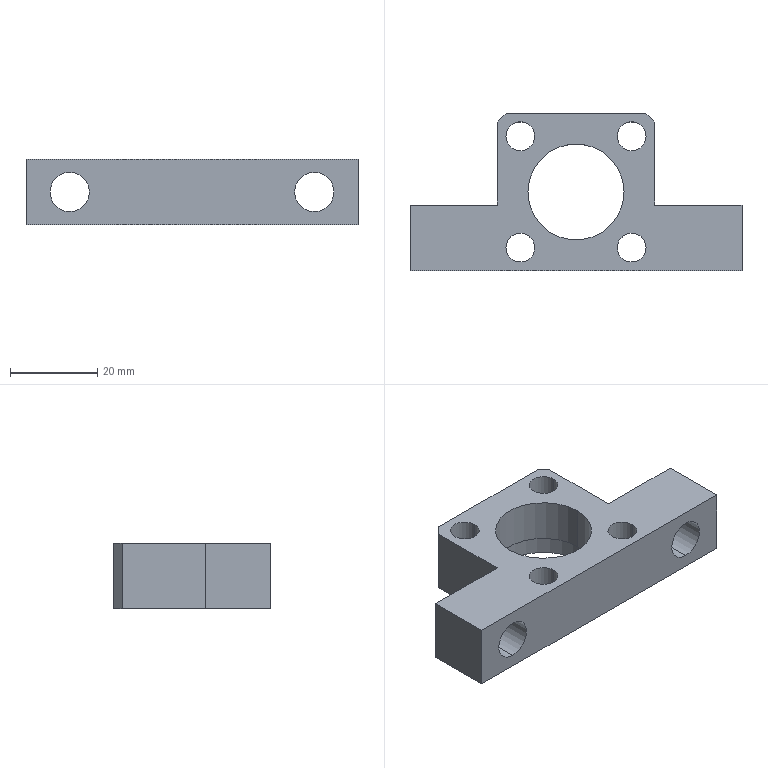Part | STEP file | 1 solid | 29 faces | box 76 x 36 x 15 mm | volume 18163 mm3 | cylinder 16 | plane 13 | commonest cylinder face diameters 6.6 x8 9 x4 22 x2 25 x2